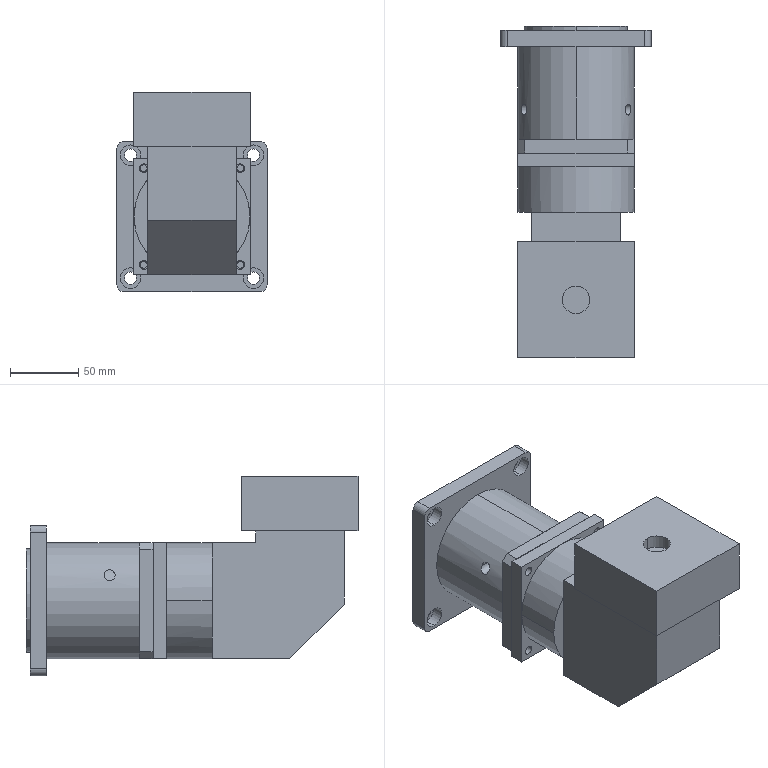Part | NX | features BREP 5 | 5 solids | 399 faces | box 110 x 243 x 146 mm | volume 1556331 mm3 | cylinder 163 | cone 111 | plane 103 | torus 22 | commonest cylinder face diameters 22.654 x18 22.734 x18 3 x16 5 x12 6.5 x12 20 x9